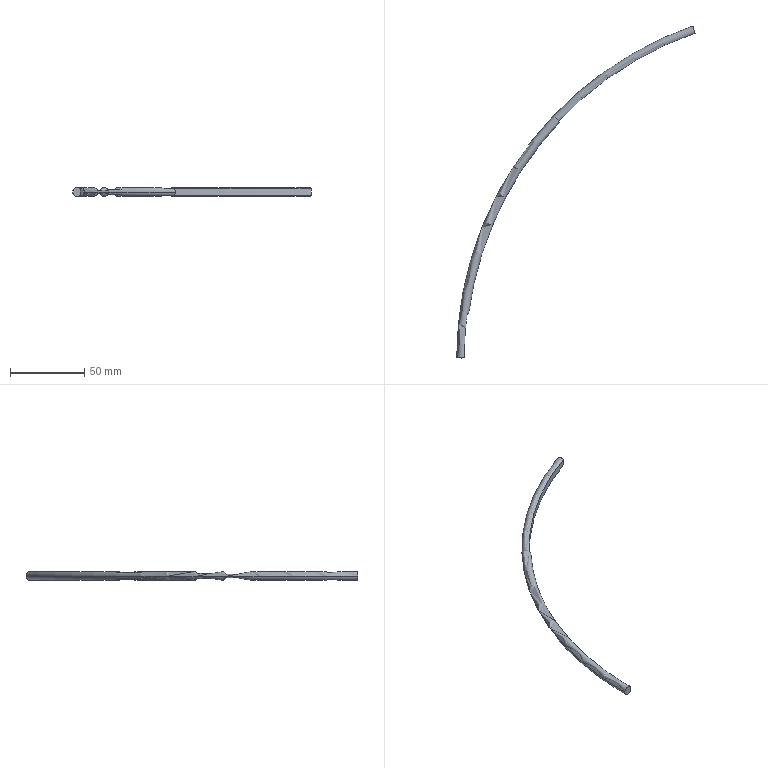Part | SolidWorks | features ICE 1, Sweep 1 | 1 solid | 8 faces | box 160.032 x 222.873 x 6 mm | volume 7707 mm3 | plane 4 | torus 2 | cylinder 2 | commonest cylinder face diameters 462 x2
STEP:
#1=CARTESIAN_POINT('',(-75.968,218.151,2.236));
#2=VERTEX_POINT('',#1);
#3=CARTESIAN_POINT('',(-77.613,222.873,0.));
#4=VERTEX_POINT('',#3);
#5=CARTESIAN_POINT('',(-76.626,220.04,0.));
#6=DIRECTION('',(-0.9444,-0.3289,0.));
#7=DIRECTION('',(0.3289,-0.9444,0.));
#8=AXIS2_PLACEMENT_3D('',#5,#6,#7);
#9=CIRCLE('',#8,3.);
#10=EDGE_CURVE('',#2,#4,#9,.T.);
#11=ORIENTED_EDGE('',*,*,#10,.T.);
#12=CARTESIAN_POINT('',(-236.,0.,0.));
#13=VERTEX_POINT('',#12);
#14=CARTESIAN_POINT('',(0.,0.,0.));
#15=DIRECTION('',(0.,0.,1.));
#16=DIRECTION('',(1.,0.,0.));
#17=AXIS2_PLACEMENT_3D('',#14,#15,#16);
#18=CIRCLE('',#17,236.);
#19=EDGE_CURVE('',#4,#13,#18,.T.);
#20=ORIENTED_EDGE('',*,*,#19,.T.);
#21=CARTESIAN_POINT('',(-231.,0.,2.236));
#22=VERTEX_POINT('',#21);
#23=CARTESIAN_POINT('',(-233.,0.,0.));
#24=DIRECTION('',(0.,-1.,0.));
#25=DIRECTION('',(1.,0.,0.));
#26=AXIS2_PLACEMENT_3D('',#23,#24,#25);
#27=CIRCLE('',#26,3.);
#28=EDGE_CURVE('',#22,#13,#27,.T.);
#29=ORIENTED_EDGE('',*,*,#28,.F.);
#30=CARTESIAN_POINT('',(-229.076,29.752,2.236));
#31=VERTEX_POINT('',#30);
#32=CARTESIAN_POINT('',(0.,0.,2.236));
#33=DIRECTION('',(0.,0.,1.));
#34=DIRECTION('',(-1.,0.,0.));
#35=AXIS2_PLACEMENT_3D('',#32,#33,#34);
#36=CIRCLE('',#35,231.);
#37=EDGE_CURVE('',#31,#22,#36,.T.);
#38=ORIENTED_EDGE('',*,*,#37,.F.);
#39=CARTESIAN_POINT('',(-228.084,29.623,0.));
#40=VERTEX_POINT('',#39);
#41=CARTESIAN_POINT('',(-231.059,30.009,0.));
#42=DIRECTION('',(-0.1288,-0.9917,0.));
#43=DIRECTION('',(-0.9917,0.1288,0.));
#44=AXIS2_PLACEMENT_3D('',#41,#42,#43);
#45=CIRCLE('',#44,3.);
#46=EDGE_CURVE('',#40,#31,#45,.T.);
#47=ORIENTED_EDGE('',*,*,#46,.F.);
#48=CARTESIAN_POINT('',(-167.112,158.03,0.));
#49=VERTEX_POINT('',#48);
#50=CARTESIAN_POINT('',(0.,0.,0.));
#51=DIRECTION('',(0.,0.,1.));
#52=DIRECTION('',(1.,0.,0.));
#53=AXIS2_PLACEMENT_3D('',#50,#51,#52);
#54=CIRCLE('',#53,230.);
#55=EDGE_CURVE('',#49,#40,#54,.T.);
#56=ORIENTED_EDGE('',*,*,#55,.F.);
#57=CARTESIAN_POINT('',(-167.839,158.717,2.236));
#58=VERTEX_POINT('',#57);
#59=CARTESIAN_POINT('',(-169.292,160.091,0.));
#60=DIRECTION('',(-0.6871,-0.7266,0.));
#61=DIRECTION('',(-0.7266,0.6871,0.));
#62=AXIS2_PLACEMENT_3D('',#59,#60,#61);
#63=CIRCLE('',#62,3.);
#64=EDGE_CURVE('',#49,#58,#63,.T.);
#65=ORIENTED_EDGE('',*,*,#64,.T.);
#66=CARTESIAN_POINT('',(0.,0.,2.236));
#67=DIRECTION('',(0.,0.,1.));
#68=DIRECTION('',(-1.,0.,0.));
#69=AXIS2_PLACEMENT_3D('',#66,#67,#68);
#70=CIRCLE('',#69,231.);
#71=EDGE_CURVE('',#2,#58,#70,.T.);
#72=ORIENTED_EDGE('',*,*,#71,.F.);
#73=EDGE_LOOP('',(#11,#20,#29,#38,#47,#56,#65,#72));
#74=FACE_OUTER_BOUND('',#73,.T.);
#75=CARTESIAN_POINT('',(0.,0.,0.));
#76=DIRECTION('',(0.,0.,1.));
#77=DIRECTION('',(1.,0.,0.));
#78=AXIS2_PLACEMENT_3D('',#75,#76,#77);
#79=TOROIDAL_SURFACE('',#78,233.,3.);
#80=ADVANCED_FACE('',(#74),#79,.T.);
#81=ORIENTED_EDGE('',*,*,#19,.F.);
#82=CARTESIAN_POINT('',(-75.968,218.151,-2.236));
#83=VERTEX_POINT('',#82);
#84=CARTESIAN_POINT('',(-76.626,220.04,0.));
#85=DIRECTION('',(-0.9444,-0.3289,0.));
#86=DIRECTION('',(0.3289,-0.9444,0.));
#87=AXIS2_PLACEMENT_3D('',#84,#85,#86);
#88=CIRCLE('',#87,3.);
#89=EDGE_CURVE('',#4,#83,#88,.T.);
#90=ORIENTED_EDGE('',*,*,#89,.T.);
#91=CARTESIAN_POINT('',(-167.839,158.717,-2.236));
#92=VERTEX_POINT('',#91);
#93=CARTESIAN_POINT('',(0.,0.,-2.236));
#94=DIRECTION('',(0.,0.,-1.));
#95=DIRECTION('',(1.,0.,0.));
#96=AXIS2_PLACEMENT_3D('',#93,#94,#95);
#97=CIRCLE('',#96,231.);
#98=EDGE_CURVE('',#92,#83,#97,.T.);
#99=ORIENTED_EDGE('',*,*,#98,.F.);
#100=CARTESIAN_POINT('',(-169.292,160.091,0.));
#101=DIRECTION('',(-0.6871,-0.7266,0.));
#102=DIRECTION('',(-0.7266,0.6871,0.));
#103=AXIS2_PLACEMENT_3D('',#100,#101,#102);
#104=CIRCLE('',#103,3.);
#105=EDGE_CURVE('',#92,#49,#104,.T.);
#106=ORIENTED_EDGE('',*,*,#105,.T.);
#107=ORIENTED_EDGE('',*,*,#55,.T.);
#108=CARTESIAN_POINT('',(-229.076,29.752,-2.236));
#109=VERTEX_POINT('',#108);
#110=CARTESIAN_POINT('',(-231.059,30.009,0.));
#111=DIRECTION('',(-0.1288,-0.9917,0.));
#112=DIRECTION('',(-0.9917,0.1288,0.));
#113=AXIS2_PLACEMENT_3D('',#110,#111,#112);
#114=CIRCLE('',#113,3.);
#115=EDGE_CURVE('',#109,#40,#114,.T.);
#116=ORIENTED_EDGE('',*,*,#115,.F.);
#117=CARTESIAN_POINT('',(-231.,0.,-2.236));
#118=VERTEX_POINT('',#117);
#119=CARTESIAN_POINT('',(0.,0.,-2.236));
#120=DIRECTION('',(0.,0.,-1.));
#121=DIRECTION('',(1.,0.,0.));
#122=AXIS2_PLACEMENT_3D('',#119,#120,#121);
#123=CIRCLE('',#122,231.);
#124=EDGE_CURVE('',#118,#109,#123,.T.);
#125=ORIENTED_EDGE('',*,*,#124,.F.);
#126=CARTESIAN_POINT('',(-233.,0.,0.));
#127=DIRECTION('',(0.,-1.,0.));
#128=DIRECTION('',(1.,0.,0.));
#129=AXIS2_PLACEMENT_3D('',#126,#127,#128);
#130=CIRCLE('',#129,3.);
#131=EDGE_CURVE('',#13,#118,#130,.T.);
#132=ORIENTED_EDGE('',*,*,#131,.F.);
#133=EDGE_LOOP('',(#81,#90,#99,#106,#107,#116,#125,#132));
#134=FACE_OUTER_BOUND('',#133,.T.);
#135=CARTESIAN_POINT('',(0.,0.,0.));
#136=DIRECTION('',(0.,0.,1.));
#137=DIRECTION('',(1.,0.,0.));
#138=AXIS2_PLACEMENT_3D('',#135,#136,#137);
#139=TOROIDAL_SURFACE('',#138,233.,3.);
#140=ADVANCED_FACE('',(#134),#139,.T.);
#141=CARTESIAN_POINT('',(-231.,0.,-25.));
#142=DIRECTION('',(0.,0.,1.));
#143=VECTOR('',#142,1000.);
#144=LINE('',#141,#143);
#145=EDGE_CURVE('',#118,#22,#144,.T.);
#146=ORIENTED_EDGE('',*,*,#145,.T.);
#147=ORIENTED_EDGE('',*,*,#28,.T.);
#148=ORIENTED_EDGE('',*,*,#131,.T.);
#149=EDGE_LOOP('',(#146,#147,#148));
#150=FACE_OUTER_BOUND('',#149,.T.);
#151=CARTESIAN_POINT('',(-233.,0.,0.));
#152=DIRECTION('',(0.,-1.,0.));
#153=DIRECTION('',(1.,0.,0.));
#154=AXIS2_PLACEMENT_3D('',#151,#152,#153);
#155=PLANE('',#154);
#156=ADVANCED_FACE('',(#150),#155,.T.);
#157=ORIENTED_EDGE('',*,*,#10,.F.);
#158=CARTESIAN_POINT('',(-75.968,218.151,-25.));
#159=DIRECTION('',(0.,0.,1.));
#160=VECTOR('',#159,1000.);
#161=LINE('',#158,#160);
#162=EDGE_CURVE('',#83,#2,#161,.T.);
#163=ORIENTED_EDGE('',*,*,#162,.F.);
#164=ORIENTED_EDGE('',*,*,#89,.F.);
#165=EDGE_LOOP('',(#157,#163,#164));
#166=FACE_OUTER_BOUND('',#165,.T.);
#167=CARTESIAN_POINT('',(-76.626,220.04,0.));
#168=DIRECTION('',(-0.9444,-0.3289,0.));
#169=DIRECTION('',(0.3289,-0.9444,0.));
#170=AXIS2_PLACEMENT_3D('',#167,#168,#169);
#171=PLANE('',#170);
#172=ADVANCED_FACE('',(#166),#171,.F.);
#173=ORIENTED_EDGE('',*,*,#115,.T.);
#174=ORIENTED_EDGE('',*,*,#46,.T.);
#175=CARTESIAN_POINT('',(-229.076,29.752,-25.));
#176=DIRECTION('',(0.,0.,1.));
#177=VECTOR('',#176,1000.);
#178=LINE('',#175,#177);
#179=EDGE_CURVE('',#109,#31,#178,.T.);
#180=ORIENTED_EDGE('',*,*,#179,.F.);
#181=EDGE_LOOP('',(#173,#174,#180));
#182=FACE_OUTER_BOUND('',#181,.T.);
#183=CARTESIAN_POINT('',(0.,0.,-25.));
#184=DIRECTION('',(0.1288,0.9917,0.));
#185=DIRECTION('',(-0.9917,0.1288,0.));
#186=AXIS2_PLACEMENT_3D('',#183,#184,#185);
#187=PLANE('',#186);
#188=ADVANCED_FACE('',(#182),#187,.F.);
#189=ORIENTED_EDGE('',*,*,#37,.T.);
#190=ORIENTED_EDGE('',*,*,#145,.F.);
#191=ORIENTED_EDGE('',*,*,#124,.T.);
#192=ORIENTED_EDGE('',*,*,#179,.T.);
#193=EDGE_LOOP('',(#189,#190,#191,#192));
#194=FACE_OUTER_BOUND('',#193,.T.);
#195=CARTESIAN_POINT('',(0.,0.,-25.));
#196=DIRECTION('',(0.,0.,1.));
#197=DIRECTION('',(1.,0.,0.));
#198=AXIS2_PLACEMENT_3D('',#195,#196,#197);
#199=CYLINDRICAL_SURFACE('',#198,231.);
#200=ADVANCED_FACE('',(#194),#199,.F.);
#201=CARTESIAN_POINT('',(-167.839,158.717,-25.));
#202=DIRECTION('',(0.,0.,1.));
#203=VECTOR('',#202,1000.);
#204=LINE('',#201,#203);
#205=EDGE_CURVE('',#92,#58,#204,.T.);
#206=ORIENTED_EDGE('',*,*,#205,.T.);
#207=ORIENTED_EDGE('',*,*,#64,.F.);
#208=ORIENTED_EDGE('',*,*,#105,.F.);
#209=EDGE_LOOP('',(#206,#207,#208));
#210=FACE_OUTER_BOUND('',#209,.T.);
#211=CARTESIAN_POINT('',(0.,0.,-25.));
#212=DIRECTION('',(0.6871,0.7266,0.));
#213=DIRECTION('',(-0.7266,0.6871,0.));
#214=AXIS2_PLACEMENT_3D('',#211,#212,#213);
#215=PLANE('',#214);
#216=ADVANCED_FACE('',(#210),#215,.T.);
#217=ORIENTED_EDGE('',*,*,#71,.T.);
#218=ORIENTED_EDGE('',*,*,#205,.F.);
#219=ORIENTED_EDGE('',*,*,#98,.T.);
#220=ORIENTED_EDGE('',*,*,#162,.T.);
#221=EDGE_LOOP('',(#217,#218,#219,#220));
#222=FACE_OUTER_BOUND('',#221,.T.);
#223=CARTESIAN_POINT('',(0.,0.,-25.));
#224=DIRECTION('',(0.,0.,1.));
#225=DIRECTION('',(1.,0.,0.));
#226=AXIS2_PLACEMENT_3D('',#223,#224,#225);
#227=CYLINDRICAL_SURFACE('',#226,231.);
#228=ADVANCED_FACE('',(#222),#227,.F.);
#229=CLOSED_SHELL('',(#80,#140,#156,#172,#188,#200,#216,#228));
#230=MANIFOLD_SOLID_BREP('',#229);
#231=CARTESIAN_POINT('',(0.,0.,0.));
#232=DIRECTION('',(0.,0.,1.));
#233=DIRECTION('',(1.,0.,0.));
#234=AXIS2_PLACEMENT_3D('',#231,#232,#233);
#235=(LENGTH_UNIT()NAMED_UNIT(*)SI_UNIT(.MILLI.,.METRE.));
#236=UNCERTAINTY_MEASURE_WITH_UNIT(LENGTH_MEASURE(0.00001),#235,'','');
#237=(NAMED_UNIT(*)PLANE_ANGLE_UNIT()SI_UNIT($,.RADIAN.));
#238=(NAMED_UNIT(*)SI_UNIT($,.STERADIAN.)SOLID_ANGLE_UNIT());
#239=(GEOMETRIC_REPRESENTATION_CONTEXT(3)GLOBAL_UNCERTAINTY_ASSIGNED_CONTEXT((#236))GLOBAL_UNIT_ASSIGNED_CONTEXT((#235,#237,#238))REPRESENTATION_CONTEXT('',''));
#240=ADVANCED_BREP_SHAPE_REPRESENTATION('',(#230,#234),#239);